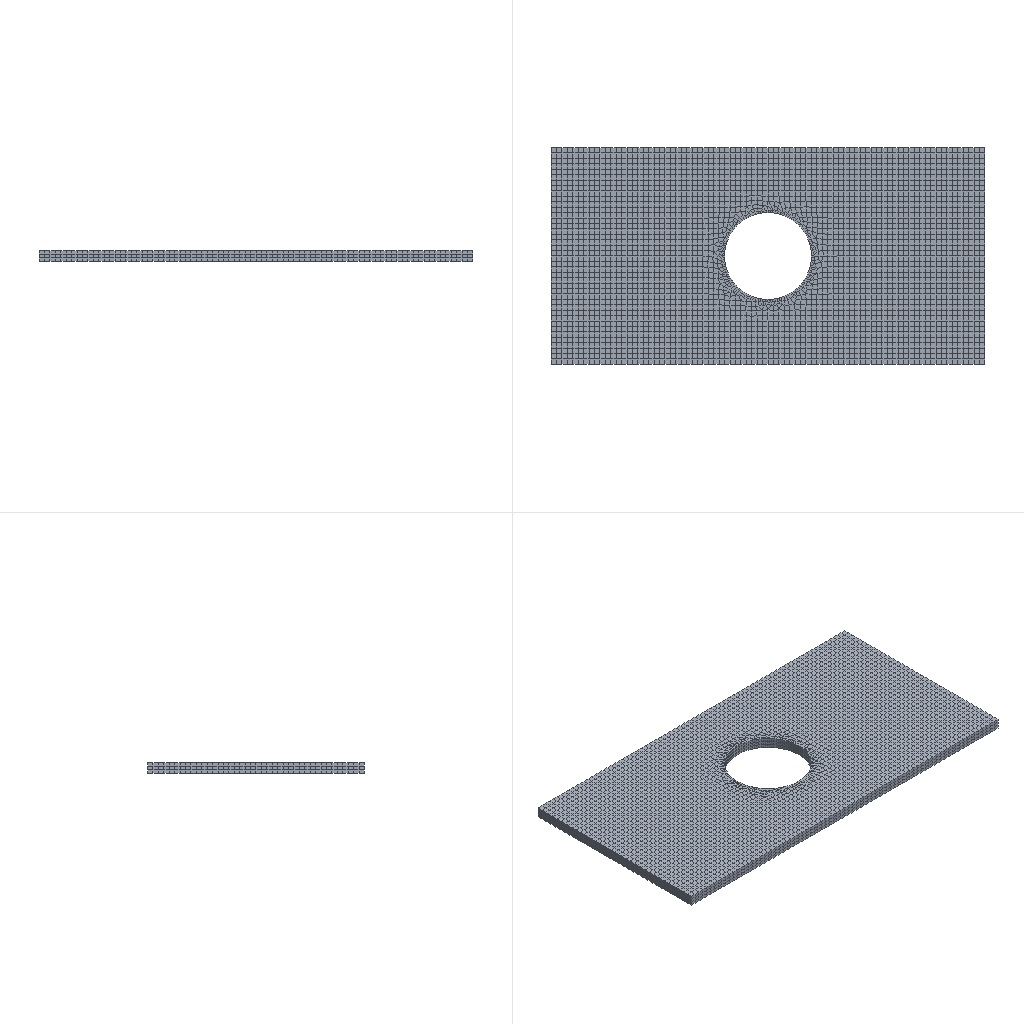Simulation study | ansys workbench
Set-up summary:
category,name,step,type,value,unit,region
solver,ansys_workbench
units,mm-N-s-tonne (MPa),,stated,"/units,MPA"
analysis,LS1,,static
load_step,LS1,LS1,static,nsubst=1; time=1
mesh,nodes,,,50096
mesh,elements,,,9861
element_type,SOLID186,,,9621
element_type,SURF154,,,240
material,Structural Steel,,E,200000,tonne s^-2 mm^-1
material,Structural Steel,,nu,0.3
material,Structural Steel,,density,7.85e-09,tonne mm^-3
material,Structural Steel,,conductivity,60.5,tonne mm s^-3 C^-1
material,Structural Steel,,specific_heat,4.34e+08,mm^2 s^-2 C^-1
material,Structural Steel,,cte,1.2e-05,C^-1
material,Structural Steel,,permeability,10000
material,Structural Steel,,resistivity,0.00017,ohm mm
load,Define Force Using Surface Effect Elements,LS1,surface-effect pres face 1,20,,SURF154 #2
load,Define Force Using Surface Effect Elements,LS1,surface-effect pres face 1,-20,,SURF154 #3
bc,Constant Zero Displacement Z,model,fixed,[dofs=UZ],,_DISPZEROUZ
named_set,_DISPZEROUZ,,node,9983
Ansys APDL input file, long lists of numbers shortened:
/batch
/config,noeldb,1     ! force off writing results to database
*get,_wallstrt,active,,time,wall
! ANSYS input file written by Workbench version 2021 R1
! File used for geometry attach:
/title,wbnew--____ (C5)
! ****** Begin Custom Load Command Snippet ******
/COM, ACT Extensions:
/COM,     LSDYNA, 2021.1
/COM,
! ****** End   Custom Load Command Snippet ******
*DIM,_wb_ProjectScratch_dir,string,248
_wb_ProjectScratch_dir(1) = ''
*DIM,_wb_SolverFiles_dir,string,248
_wb_SolverFiles_dir(1) = ''
*DIM,_wb_userfiles_dir,string,248
_wb_userfiles_dir(1) = ''
/com,--- Data in consistent NMM units. See Solving Units in the help system for more information.
/units,MPA
/nopr
/wb,file,start              !  signify a WB generated input file
/prep7
! Turn off shape checking because checks already performed inside WB mesher.
! See help system for more information.
SHPP,OFF,,NOWARN
/nolist
etcon,set             ! allow ANSYS to choose best KEYOP's for 180x elements, resets any applicable keyopt to MAPDL defaults
/com,*********** Nodes for the whole assembly ***********
nblock,3,,55105
(1i9,3e20.9e3)
        1     2.054137425E+01     2.480235324E+00     1.666666667E+00
! (50095 more lines like these left out)
-1
/wb,elem,start            !  set before creation of elements
/com,*********** Elements for Body 1 "2-FreeParts|____-____1" ***********
et,1,186
keyo,1,2,1          ! set full integration on SOLID186
eblock,19,solid,,9621
(19i9)
        1        1        1        1        0        0        0        0       20        0        1        1        3     3873     3871     9066     9065     7130     7131
! (19241 more lines like these left out)
-1
/wb,elem,end               !  done creating elements
/com,*********** Send User Defined Coordinate System(s) ***********
csys,0
toffst,273.15,  ! Temperature offset from absolute zero
/com,*********** Set Reference Temperature ***********
tref,22.
/wb,mat,start              !  starting to send materials
/com,*********** Send Materials ***********
Temperature = 'TEMP' ! Temperature
MP,DENS,1,7.85e-09,	! tonne mm^-3
MP,ALPX,1,1.2e-05,	! C^-1
MP,C,1,434000000,	! mm^2 s^-2 C^-1
MP,KXX,1,60.5,	! tonne mm s^-3 C^-1
MP,RSVX,1,0.00017,	! ohm mm
MP,EX,1,200000,	! tonne s^-2 mm^-1
MP,NUXY,1,0.3,
MP,MURX,1,10000,
/wb,mat,end                !  done sending materials
!************************* Model Summary ********************
!2-FreeParts|____-____1,	结构钢,	matid,	1
!************************* End Model Summary ********************
! get the diagonal of the bounding box. Needed later for other things
*get,_xmin,node,,mnloc,x
*get,_ymin,node,,mnloc,y
*get,_zmin,node,,mnloc,z
*get,_xmax,node,,mxloc,x
*get,_ymax,node,,mxloc,y
*get,_zmax,node,,mxloc,z
_ASMDIAG=(_xmax-_xmin)*(_xmax-_xmin)+(_ymax-_ymin)*(_ymax-_ymin)+(_zmax-_zmin)*(_zmax-_zmin)
_ASMDIAG=SQRT(_ASMDIAG)
/wb,contact,start          !  starting to send contact
/wb,contact,end            !  done creating contacts
/golist
/wb,load,start             !  starting to send loads
/com,******* Constant Zero Displacement Z *******
CMBLOCK,_DISPZEROUZ,NODE,     9983
(8i10)
      6045      6046      6047      6048      6049      6050      6051      6052
! (1247 more lines like these left out)
cmsel,s,_DISPZEROUZ
d,all,uz,0
nsel,all
/com,*********** Define Force Using Surface Effect Elements ***********
local,12,0,0.,0.,0.,0.,0.,0.
csys,0
et,2,154
eblock,10,,,120
(15i9)
    17134        2        2        2       12    13008    12890    13006    13007    49001    49000    49192    49193
! (119 more lines like these left out)
-1
esel,s,type,,2
keyop,2,2,1                ! Apply load in local coordinate system
keyop,2,7,1                ! Use original area so load is constant in large deformation
esel,all
/com,*********** Define Force Using Surface Effect Elements ***********
local,13,0,0.,0.,0.,0.,0.,0.
csys,0
et,3,154
eblock,10,,,120
(15i9)
    17254        3        3        3       13    13249    13436    12089    12269    49597    47537    47536    47898
! (119 more lines like these left out)
-1
esel,s,type,,3
keyop,3,2,1                ! Apply load in local coordinate system
keyop,3,7,1                ! Use original area so load is constant in large deformation
esel,all
/gst,on,on
fini
*get,_numnode,node,0,count
*get,_numelem,elem,0,count
*get, _MAXELEMNUM, elem, 0, NUM, MAX
*get, _MAXNODENUM, node, 0, NUM, MAX
*get, _MAXELEMTYPE, etyp, 0, NUM, MAX
*get, _MAXREALCONST, real, 0, NUM, MAX
/go
/wb,load,end               !  done creating loads
/com,--- Number of total nodes = %_numnode%
/com,--- Number of contact elements = 240
/com,--- Number of spring elements = 0
/com,--- Number of bearing elements = 0
/com,--- Number of solid elements = 9621
/com,--- Number of condensed parts = 0
/com,--- Number of total elements = %_numelem%
*get,_wallbsol,active,,time,wall
/com,****************************************************************************
/com,*************************    SOLUTION       ********************************
/com,****************************************************************************
/solu
antype,0                   ! static analysis
_thickRatio=  1     ! Ratio of thick parts in the model
eqsl,pcg,1e-8,,,,,,1
cntr,print,1               ! print out contact info and also make no initial contact an error
dmpoption,emat,no             ! Don't combine emat file for DANSYS
dmpoption,esav,no             ! Don't combine esav file for DANSYS
nldiag,cont,iter           ! print out contact info each equilibrium iteration
rescontrol,,none                 ! Do not keep any restart files
/com,****************************************************
/com,******************* SOLVE FOR LS 1 OF 1 ****************
esel,s,type,,2
nsle
sfe,all,1,pres,1,20.
sfe,all,2,pres,1,0.
sfe,all,3,pres,1,0.
esel,s,type,,3
nsle
sfe,all,1,pres,1,-20.
sfe,all,2,pres,1,0.
sfe,all,3,pres,1,0.
nsel,all
esel,all
/nopr
/gopr
/nolist
nsub,1,1,1
time,1.
outres,erase
outres,all,none
outres,nsol,all,
outres,rsol,all
outres,eangl,all
outres,etmp,all
outres,veng,all
outres,strs,all,
outres,epel,all,
outres,eppl,all,
outres,cont,all,
! *********** WB SOLVE COMMAND ***********
! check interactive state
*get,ANSINTER_,active,,int
*if,ANSINTER_,ne,0,then
/eof
*endif
solve
/com *************** Write FE CONNECTORS *********
CEWRITE,file,ce,,INTE
/com,****************************************************
/com,*************** FINISHED SOLVE FOR LS 1 *************
*get,_wallasol,active,,time,wall
/nopr
*get,_numnode,node,0,count
*get,_numelem,elem,0,count
*get, _MAXELEMNUM, elem, 0, NUM, MAX
*get, _MAXNODENUM, node, 0, NUM, MAX,,,INTERNAL
*get, _MAXELEMTYPE, etyp, 0, NUM, MAX
*get, _MAXREALCONST, real, 0, NUM, MAX
/gopr
*get,_PCGITER,active,,solu,cgiter
/post1
xmlo,ENCODING,ISO-8859-1
xmlo,parm
/xml,parm,xml
fini
/gopr
*get,_walldone,active,,time,wall
_preptime=(_wallbsol-_wallstrt)*3600
_solvtime=(_wallasol-_wallbsol)*3600
_posttime=(_walldone-_wallasol)*3600
_totaltim=(_walldone-_wallstrt)*3600
*get,_dlbratio,active,0,solu,dlbr
*get,_combtime,active,0,solu,comb
/com,--- Total number of nodes = %_numnode%
/com,--- Total number of elements = %_numelem%
/com,--- Element load balance ratio = %_dlbratio%
/com,--- Time to combine distributed files = %_combtime%
/wb,file,end               ! done with WB generated input
Results summary:
result,analyses[0].index,,,1
result,analyses[0].system,,,SYS-2
result,analyses[0].deck,,,deck.dat
result,analyses[0].solve_status,,,completed
result,analyses[0].analysis_type,,,static
result,analyses[0].physics,,,mechanical
result,analyses[0].unit_system,,,"NMM: mm, ton, N, s, mV, mA, degC"
result,analyses[0].n_sets,,,1
result,analyses[0].load_steps[0].set,set=1,,1
result,analyses[0].load_steps[0].time_or_freq,set=1,,1
result,analyses[0].load_steps[0].max_displacement_magnitude,set=1,,0.5424
result,analyses[0].load_steps[0].max_von_mises_nodal,set=1,,75.686
result,analyses[0].load_steps[0].reaction_force_sum_xyz[1],set=1,,0
result,analyses[0].load_steps[0].reaction_force_sum_xyz[2],set=1,,0
result,analyses[0].load_steps[0].reaction_force_sum_xyz[3],set=1,,9.11286e-05
result,geometry_export[0][0],,,.step
result,geometry_export[0][1],,,ok
result,geometry_export[0][2],,,1